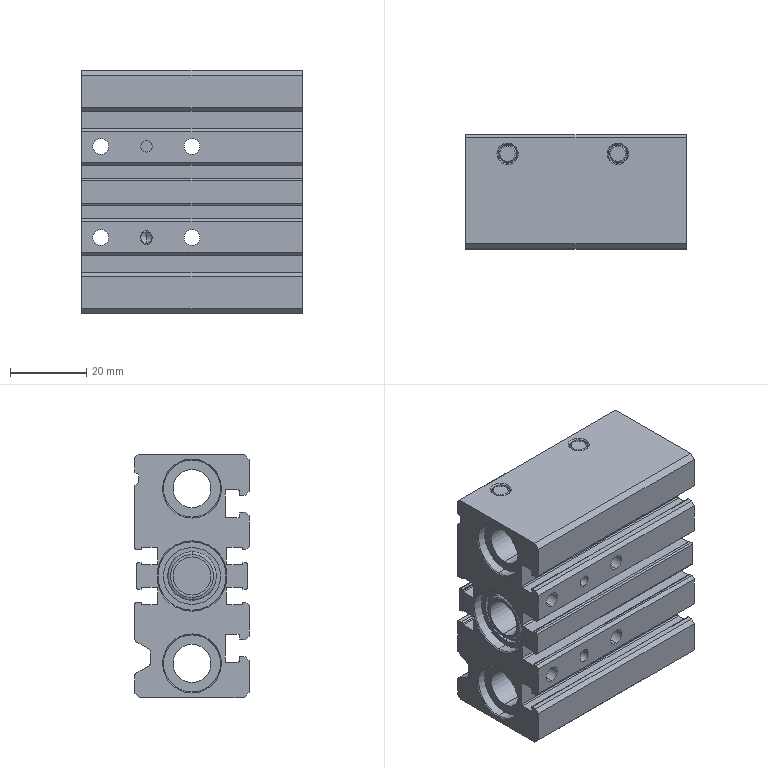Part | STEP file | 11-_TC-M-16x2525_b11 | 1 solid | 297 faces | box 58 x 30 x 64 mm | volume 71098 mm3 | cylinder 130 | plane 101 | cone 64 | spline 2 | commonest cylinder face diameters 0.8 x20 4.134 x20 0.4 x16 3 x14 4.5 x8 8 x8